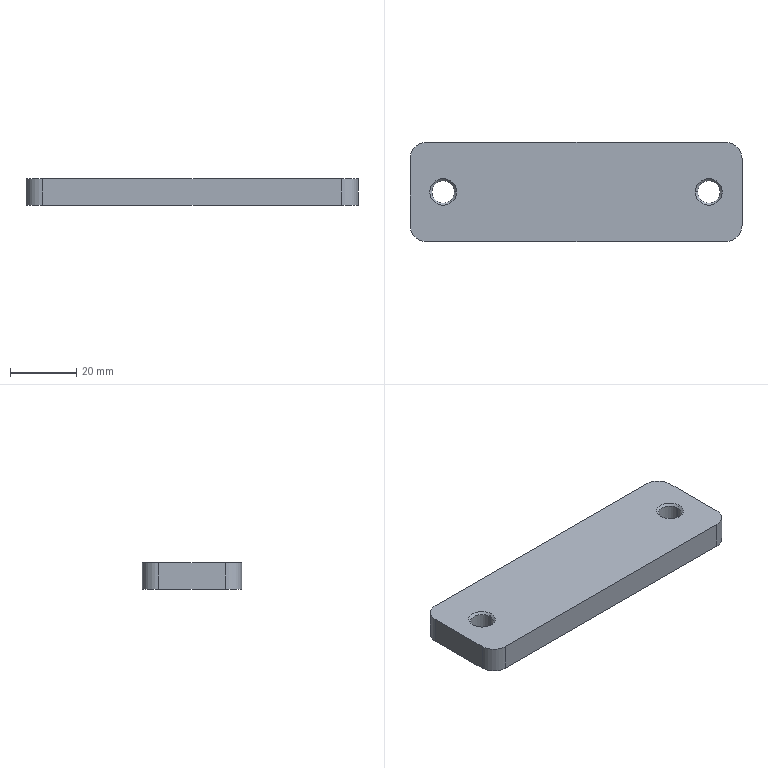Part | SolidWorks | features Extrusion 1, Fillet 1, HoleWzd 1 | 1 solid | 18 faces | box 100 x 30 x 8 mm | volume 23238 mm3 | cylinder 8 | plane 6 | cone 4 | commonest cylinder face diameters 6.8 x4 10 x4
STEP:
#1=CARTESIAN_POINT('',(-43.4,0.,7.375));
#2=VERTEX_POINT('',#1);
#3=CARTESIAN_POINT('',(-36.6,0.,7.375));
#4=VERTEX_POINT('',#3);
#5=CARTESIAN_POINT('',(-40.,0.,7.375));
#6=DIRECTION('',(0.,0.,1.));
#7=DIRECTION('',(1.,0.,0.));
#8=AXIS2_PLACEMENT_3D('',#5,#6,#7);
#9=CIRCLE('',#8,3.4);
#10=EDGE_CURVE('',#2,#4,#9,.T.);
#11=ORIENTED_EDGE('',*,*,#10,.F.);
#12=CARTESIAN_POINT('',(-44.025,0.,8.));
#13=VERTEX_POINT('',#12);
#14=CARTESIAN_POINT('',(-44.025,0.,8.));
#15=DIRECTION('',(-0.7071,0.,0.7071));
#16=VECTOR('',#15,1000.);
#17=LINE('',#14,#16);
#18=EDGE_CURVE('',#2,#13,#17,.T.);
#19=ORIENTED_EDGE('',*,*,#18,.T.);
#20=CARTESIAN_POINT('',(-35.975,0.,8.));
#21=VERTEX_POINT('',#20);
#22=CARTESIAN_POINT('',(-40.,0.,8.));
#23=DIRECTION('',(0.,0.,1.));
#24=DIRECTION('',(1.,0.,0.));
#25=AXIS2_PLACEMENT_3D('',#22,#23,#24);
#26=CIRCLE('',#25,4.025);
#27=EDGE_CURVE('',#13,#21,#26,.T.);
#28=ORIENTED_EDGE('',*,*,#27,.T.);
#29=CARTESIAN_POINT('',(-35.975,0.,8.));
#30=DIRECTION('',(0.7071,0.,0.7071));
#31=VECTOR('',#30,1000.);
#32=LINE('',#29,#31);
#33=EDGE_CURVE('',#4,#21,#32,.T.);
#34=ORIENTED_EDGE('',*,*,#33,.F.);
#35=EDGE_LOOP('',(#11,#19,#28,#34));
#36=FACE_OUTER_BOUND('',#35,.T.);
#37=CARTESIAN_POINT('',(-40.,0.,8.));
#38=DIRECTION('',(0.,0.,1.));
#39=DIRECTION('',(1.,0.,0.));
#40=AXIS2_PLACEMENT_3D('',#37,#38,#39);
#41=CONICAL_SURFACE('',#40,4.025,0.7854);
#42=ADVANCED_FACE('',(#36),#41,.F.);
#43=CARTESIAN_POINT('',(-43.4,0.,0.));
#44=VERTEX_POINT('',#43);
#45=CARTESIAN_POINT('',(-36.6,0.,0.));
#46=VERTEX_POINT('',#45);
#47=CARTESIAN_POINT('',(-40.,0.,0.));
#48=DIRECTION('',(0.,0.,1.));
#49=DIRECTION('',(1.,0.,0.));
#50=AXIS2_PLACEMENT_3D('',#47,#48,#49);
#51=CIRCLE('',#50,3.4);
#52=EDGE_CURVE('',#44,#46,#51,.T.);
#53=ORIENTED_EDGE('',*,*,#52,.F.);
#54=CARTESIAN_POINT('',(-43.4,0.,8.));
#55=DIRECTION('',(0.,0.,1.));
#56=VECTOR('',#55,1000.);
#57=LINE('',#54,#56);
#58=EDGE_CURVE('',#44,#2,#57,.T.);
#59=ORIENTED_EDGE('',*,*,#58,.T.);
#60=ORIENTED_EDGE('',*,*,#10,.T.);
#61=CARTESIAN_POINT('',(-36.6,0.,8.));
#62=DIRECTION('',(0.,0.,1.));
#63=VECTOR('',#62,1000.);
#64=LINE('',#61,#63);
#65=EDGE_CURVE('',#46,#4,#64,.T.);
#66=ORIENTED_EDGE('',*,*,#65,.F.);
#67=EDGE_LOOP('',(#53,#59,#60,#66));
#68=FACE_OUTER_BOUND('',#67,.T.);
#69=CARTESIAN_POINT('',(-40.,0.,8.));
#70=DIRECTION('',(0.,0.,1.));
#71=DIRECTION('',(1.,0.,0.));
#72=AXIS2_PLACEMENT_3D('',#69,#70,#71);
#73=CYLINDRICAL_SURFACE('',#72,3.4);
#74=ADVANCED_FACE('',(#68),#73,.F.);
#75=CARTESIAN_POINT('',(36.6,0.,7.375));
#76=VERTEX_POINT('',#75);
#77=CARTESIAN_POINT('',(43.4,0.,7.375));
#78=VERTEX_POINT('',#77);
#79=CARTESIAN_POINT('',(40.,0.,7.375));
#80=DIRECTION('',(0.,0.,1.));
#81=DIRECTION('',(1.,0.,0.));
#82=AXIS2_PLACEMENT_3D('',#79,#80,#81);
#83=CIRCLE('',#82,3.4);
#84=EDGE_CURVE('',#76,#78,#83,.T.);
#85=ORIENTED_EDGE('',*,*,#84,.F.);
#86=CARTESIAN_POINT('',(35.975,0.,8.));
#87=VERTEX_POINT('',#86);
#88=CARTESIAN_POINT('',(35.975,0.,8.));
#89=DIRECTION('',(-0.7071,0.,0.7071));
#90=VECTOR('',#89,1000.);
#91=LINE('',#88,#90);
#92=EDGE_CURVE('',#76,#87,#91,.T.);
#93=ORIENTED_EDGE('',*,*,#92,.T.);
#94=CARTESIAN_POINT('',(44.025,0.,8.));
#95=VERTEX_POINT('',#94);
#96=CARTESIAN_POINT('',(40.,0.,8.));
#97=DIRECTION('',(0.,0.,1.));
#98=DIRECTION('',(1.,0.,0.));
#99=AXIS2_PLACEMENT_3D('',#96,#97,#98);
#100=CIRCLE('',#99,4.025);
#101=EDGE_CURVE('',#87,#95,#100,.T.);
#102=ORIENTED_EDGE('',*,*,#101,.T.);
#103=CARTESIAN_POINT('',(44.025,0.,8.));
#104=DIRECTION('',(0.7071,0.,0.7071));
#105=VECTOR('',#104,1000.);
#106=LINE('',#103,#105);
#107=EDGE_CURVE('',#78,#95,#106,.T.);
#108=ORIENTED_EDGE('',*,*,#107,.F.);
#109=EDGE_LOOP('',(#85,#93,#102,#108));
#110=FACE_OUTER_BOUND('',#109,.T.);
#111=CARTESIAN_POINT('',(40.,0.,8.));
#112=DIRECTION('',(0.,0.,1.));
#113=DIRECTION('',(1.,0.,0.));
#114=AXIS2_PLACEMENT_3D('',#111,#112,#113);
#115=CONICAL_SURFACE('',#114,4.025,0.7854);
#116=ADVANCED_FACE('',(#110),#115,.F.);
#117=CARTESIAN_POINT('',(36.6,0.,0.));
#118=VERTEX_POINT('',#117);
#119=CARTESIAN_POINT('',(43.4,0.,0.));
#120=VERTEX_POINT('',#119);
#121=CARTESIAN_POINT('',(40.,0.,0.));
#122=DIRECTION('',(0.,0.,1.));
#123=DIRECTION('',(1.,0.,0.));
#124=AXIS2_PLACEMENT_3D('',#121,#122,#123);
#125=CIRCLE('',#124,3.4);
#126=EDGE_CURVE('',#118,#120,#125,.T.);
#127=ORIENTED_EDGE('',*,*,#126,.F.);
#128=CARTESIAN_POINT('',(36.6,0.,8.));
#129=DIRECTION('',(0.,0.,1.));
#130=VECTOR('',#129,1000.);
#131=LINE('',#128,#130);
#132=EDGE_CURVE('',#118,#76,#131,.T.);
#133=ORIENTED_EDGE('',*,*,#132,.T.);
#134=ORIENTED_EDGE('',*,*,#84,.T.);
#135=CARTESIAN_POINT('',(43.4,0.,8.));
#136=DIRECTION('',(0.,0.,1.));
#137=VECTOR('',#136,1000.);
#138=LINE('',#135,#137);
#139=EDGE_CURVE('',#120,#78,#138,.T.);
#140=ORIENTED_EDGE('',*,*,#139,.F.);
#141=EDGE_LOOP('',(#127,#133,#134,#140));
#142=FACE_OUTER_BOUND('',#141,.T.);
#143=CARTESIAN_POINT('',(40.,0.,8.));
#144=DIRECTION('',(0.,0.,1.));
#145=DIRECTION('',(1.,0.,0.));
#146=AXIS2_PLACEMENT_3D('',#143,#144,#145);
#147=CYLINDRICAL_SURFACE('',#146,3.4);
#148=ADVANCED_FACE('',(#142),#147,.F.);
#149=CARTESIAN_POINT('',(50.,-10.,8.));
#150=VERTEX_POINT('',#149);
#151=CARTESIAN_POINT('',(50.,10.,8.));
#152=VERTEX_POINT('',#151);
#153=CARTESIAN_POINT('',(50.,-15.,8.));
#154=DIRECTION('',(0.,1.,0.));
#155=VECTOR('',#154,1000.);
#156=LINE('',#153,#155);
#157=EDGE_CURVE('',#150,#152,#156,.T.);
#158=ORIENTED_EDGE('',*,*,#157,.F.);
#159=CARTESIAN_POINT('',(50.,-10.,0.));
#160=VERTEX_POINT('',#159);
#161=CARTESIAN_POINT('',(50.,-10.,8.));
#162=DIRECTION('',(0.,0.,-1.));
#163=VECTOR('',#162,1000.);
#164=LINE('',#161,#163);
#165=EDGE_CURVE('',#150,#160,#164,.T.);
#166=ORIENTED_EDGE('',*,*,#165,.T.);
#167=CARTESIAN_POINT('',(50.,10.,0.));
#168=VERTEX_POINT('',#167);
#169=CARTESIAN_POINT('',(50.,-15.,0.));
#170=DIRECTION('',(0.,1.,0.));
#171=VECTOR('',#170,1000.);
#172=LINE('',#169,#171);
#173=EDGE_CURVE('',#160,#168,#172,.T.);
#174=ORIENTED_EDGE('',*,*,#173,.T.);
#175=CARTESIAN_POINT('',(50.,10.,8.));
#176=DIRECTION('',(0.,0.,1.));
#177=VECTOR('',#176,1000.);
#178=LINE('',#175,#177);
#179=EDGE_CURVE('',#168,#152,#178,.T.);
#180=ORIENTED_EDGE('',*,*,#179,.T.);
#181=EDGE_LOOP('',(#158,#166,#174,#180));
#182=FACE_OUTER_BOUND('',#181,.T.);
#183=CARTESIAN_POINT('',(50.,-15.,8.));
#184=DIRECTION('',(-1.,0.,0.));
#185=DIRECTION('',(0.,0.,1.));
#186=AXIS2_PLACEMENT_3D('',#183,#184,#185);
#187=PLANE('',#186);
#188=ADVANCED_FACE('',(#182),#187,.F.);
#189=CARTESIAN_POINT('',(45.,15.,8.));
#190=VERTEX_POINT('',#189);
#191=CARTESIAN_POINT('',(-45.,15.,8.));
#192=VERTEX_POINT('',#191);
#193=CARTESIAN_POINT('',(-50.,15.,8.));
#194=DIRECTION('',(-1.,0.,0.));
#195=VECTOR('',#194,1000.);
#196=LINE('',#193,#195);
#197=EDGE_CURVE('',#190,#192,#196,.T.);
#198=ORIENTED_EDGE('',*,*,#197,.F.);
#199=CARTESIAN_POINT('',(45.,15.,0.));
#200=VERTEX_POINT('',#199);
#201=CARTESIAN_POINT('',(45.,15.,8.));
#202=DIRECTION('',(0.,0.,-1.));
#203=VECTOR('',#202,1000.);
#204=LINE('',#201,#203);
#205=EDGE_CURVE('',#190,#200,#204,.T.);
#206=ORIENTED_EDGE('',*,*,#205,.T.);
#207=CARTESIAN_POINT('',(-45.,15.,0.));
#208=VERTEX_POINT('',#207);
#209=CARTESIAN_POINT('',(-50.,15.,0.));
#210=DIRECTION('',(-1.,0.,0.));
#211=VECTOR('',#210,1000.);
#212=LINE('',#209,#211);
#213=EDGE_CURVE('',#200,#208,#212,.T.);
#214=ORIENTED_EDGE('',*,*,#213,.T.);
#215=CARTESIAN_POINT('',(-45.,15.,8.));
#216=DIRECTION('',(0.,0.,1.));
#217=VECTOR('',#216,1000.);
#218=LINE('',#215,#217);
#219=EDGE_CURVE('',#208,#192,#218,.T.);
#220=ORIENTED_EDGE('',*,*,#219,.T.);
#221=EDGE_LOOP('',(#198,#206,#214,#220));
#222=FACE_OUTER_BOUND('',#221,.T.);
#223=CARTESIAN_POINT('',(-50.,15.,8.));
#224=DIRECTION('',(0.,-1.,0.));
#225=DIRECTION('',(0.,0.,-1.));
#226=AXIS2_PLACEMENT_3D('',#223,#224,#225);
#227=PLANE('',#226);
#228=ADVANCED_FACE('',(#222),#227,.F.);
#229=CARTESIAN_POINT('',(-50.,10.,0.));
#230=VERTEX_POINT('',#229);
#231=CARTESIAN_POINT('',(-50.,-10.,0.));
#232=VERTEX_POINT('',#231);
#233=CARTESIAN_POINT('',(-50.,-15.,0.));
#234=DIRECTION('',(0.,-1.,0.));
#235=VECTOR('',#234,1000.);
#236=LINE('',#233,#235);
#237=EDGE_CURVE('',#230,#232,#236,.T.);
#238=ORIENTED_EDGE('',*,*,#237,.T.);
#239=CARTESIAN_POINT('',(-50.,-10.,8.));
#240=VERTEX_POINT('',#239);
#241=CARTESIAN_POINT('',(-50.,-10.,8.));
#242=DIRECTION('',(0.,0.,1.));
#243=VECTOR('',#242,1000.);
#244=LINE('',#241,#243);
#245=EDGE_CURVE('',#232,#240,#244,.T.);
#246=ORIENTED_EDGE('',*,*,#245,.T.);
#247=CARTESIAN_POINT('',(-50.,10.,8.));
#248=VERTEX_POINT('',#247);
#249=CARTESIAN_POINT('',(-50.,-15.,8.));
#250=DIRECTION('',(0.,-1.,0.));
#251=VECTOR('',#250,1000.);
#252=LINE('',#249,#251);
#253=EDGE_CURVE('',#248,#240,#252,.T.);
#254=ORIENTED_EDGE('',*,*,#253,.F.);
#255=CARTESIAN_POINT('',(-50.,10.,8.));
#256=DIRECTION('',(0.,0.,-1.));
#257=VECTOR('',#256,1000.);
#258=LINE('',#255,#257);
#259=EDGE_CURVE('',#248,#230,#258,.T.);
#260=ORIENTED_EDGE('',*,*,#259,.T.);
#261=EDGE_LOOP('',(#238,#246,#254,#260));
#262=FACE_OUTER_BOUND('',#261,.T.);
#263=CARTESIAN_POINT('',(-50.,-15.,8.));
#264=DIRECTION('',(1.,0.,0.));
#265=DIRECTION('',(0.,0.,-1.));
#266=AXIS2_PLACEMENT_3D('',#263,#264,#265);
#267=PLANE('',#266);
#268=ADVANCED_FACE('',(#262),#267,.F.);
#269=CARTESIAN_POINT('',(-45.,-15.,0.));
#270=VERTEX_POINT('',#269);
#271=CARTESIAN_POINT('',(45.,-15.,0.));
#272=VERTEX_POINT('',#271);
#273=CARTESIAN_POINT('',(-50.,-15.,0.));
#274=DIRECTION('',(1.,0.,0.));
#275=VECTOR('',#274,1000.);
#276=LINE('',#273,#275);
#277=EDGE_CURVE('',#270,#272,#276,.T.);
#278=ORIENTED_EDGE('',*,*,#277,.T.);
#279=CARTESIAN_POINT('',(45.,-15.,8.));
#280=VERTEX_POINT('',#279);
#281=CARTESIAN_POINT('',(45.,-15.,8.));
#282=DIRECTION('',(0.,0.,1.));
#283=VECTOR('',#282,1000.);
#284=LINE('',#281,#283);
#285=EDGE_CURVE('',#272,#280,#284,.T.);
#286=ORIENTED_EDGE('',*,*,#285,.T.);
#287=CARTESIAN_POINT('',(-45.,-15.,8.));
#288=VERTEX_POINT('',#287);
#289=CARTESIAN_POINT('',(-50.,-15.,8.));
#290=DIRECTION('',(1.,0.,0.));
#291=VECTOR('',#290,1000.);
#292=LINE('',#289,#291);
#293=EDGE_CURVE('',#288,#280,#292,.T.);
#294=ORIENTED_EDGE('',*,*,#293,.F.);
#295=CARTESIAN_POINT('',(-45.,-15.,8.));
#296=DIRECTION('',(0.,0.,-1.));
#297=VECTOR('',#296,1000.);
#298=LINE('',#295,#297);
#299=EDGE_CURVE('',#288,#270,#298,.T.);
#300=ORIENTED_EDGE('',*,*,#299,.T.);
#301=EDGE_LOOP('',(#278,#286,#294,#300));
#302=FACE_OUTER_BOUND('',#301,.T.);
#303=CARTESIAN_POINT('',(-50.,-15.,8.));
#304=DIRECTION('',(0.,1.,0.));
#305=DIRECTION('',(0.,0.,1.));
#306=AXIS2_PLACEMENT_3D('',#303,#304,#305);
#307=PLANE('',#306);
#308=ADVANCED_FACE('',(#302),#307,.F.);
#309=CARTESIAN_POINT('',(-40.,0.,8.));
#310=DIRECTION('',(0.,0.,1.));
#311=DIRECTION('',(1.,0.,0.));
#312=AXIS2_PLACEMENT_3D('',#309,#310,#311);
#313=CIRCLE('',#312,4.025);
#314=EDGE_CURVE('',#21,#13,#313,.T.);
#315=ORIENTED_EDGE('',*,*,#314,.F.);
#316=ORIENTED_EDGE('',*,*,#27,.F.);
#317=EDGE_LOOP('',(#315,#316));
#318=FACE_BOUND('',#317,.T.);
#319=CARTESIAN_POINT('',(40.,0.,8.));
#320=DIRECTION('',(0.,0.,1.));
#321=DIRECTION('',(1.,0.,0.));
#322=AXIS2_PLACEMENT_3D('',#319,#320,#321);
#323=CIRCLE('',#322,4.025);
#324=EDGE_CURVE('',#95,#87,#323,.T.);
#325=ORIENTED_EDGE('',*,*,#324,.F.);
#326=ORIENTED_EDGE('',*,*,#101,.F.);
#327=EDGE_LOOP('',(#325,#326));
#328=FACE_BOUND('',#327,.T.);
#329=ORIENTED_EDGE('',*,*,#293,.T.);
#330=CARTESIAN_POINT('',(45.,-10.,8.));
#331=DIRECTION('',(0.,0.,1.));
#332=DIRECTION('',(-1.,0.,0.));
#333=AXIS2_PLACEMENT_3D('',#330,#331,#332);
#334=CIRCLE('',#333,5.);
#335=EDGE_CURVE('',#280,#150,#334,.T.);
#336=ORIENTED_EDGE('',*,*,#335,.T.);
#337=ORIENTED_EDGE('',*,*,#157,.T.);
#338=CARTESIAN_POINT('',(45.,10.,8.));
#339=DIRECTION('',(0.,0.,1.));
#340=DIRECTION('',(-1.,0.,0.));
#341=AXIS2_PLACEMENT_3D('',#338,#339,#340);
#342=CIRCLE('',#341,5.);
#343=EDGE_CURVE('',#152,#190,#342,.T.);
#344=ORIENTED_EDGE('',*,*,#343,.T.);
#345=ORIENTED_EDGE('',*,*,#197,.T.);
#346=CARTESIAN_POINT('',(-45.,10.,8.));
#347=DIRECTION('',(0.,0.,1.));
#348=DIRECTION('',(-1.,0.,0.));
#349=AXIS2_PLACEMENT_3D('',#346,#347,#348);
#350=CIRCLE('',#349,5.);
#351=EDGE_CURVE('',#192,#248,#350,.T.);
#352=ORIENTED_EDGE('',*,*,#351,.T.);
#353=ORIENTED_EDGE('',*,*,#253,.T.);
#354=CARTESIAN_POINT('',(-45.,-10.,8.));
#355=DIRECTION('',(0.,0.,1.));
#356=DIRECTION('',(-1.,0.,0.));
#357=AXIS2_PLACEMENT_3D('',#354,#355,#356);
#358=CIRCLE('',#357,5.);
#359=EDGE_CURVE('',#240,#288,#358,.T.);
#360=ORIENTED_EDGE('',*,*,#359,.T.);
#361=EDGE_LOOP('',(#329,#336,#337,#344,#345,#352,#353,#360));
#362=FACE_OUTER_BOUND('',#361,.T.);
#363=CARTESIAN_POINT('',(0.,0.,8.));
#364=DIRECTION('',(0.,0.,-1.));
#365=DIRECTION('',(-1.,0.,0.));
#366=AXIS2_PLACEMENT_3D('',#363,#364,#365);
#367=PLANE('',#366);
#368=ADVANCED_FACE('',(#318,#328,#362),#367,.F.);
#369=CARTESIAN_POINT('',(-40.,0.,0.));
#370=DIRECTION('',(0.,0.,1.));
#371=DIRECTION('',(1.,0.,0.));
#372=AXIS2_PLACEMENT_3D('',#369,#370,#371);
#373=CIRCLE('',#372,3.4);
#374=EDGE_CURVE('',#46,#44,#373,.T.);
#375=ORIENTED_EDGE('',*,*,#374,.T.);
#376=ORIENTED_EDGE('',*,*,#52,.T.);
#377=EDGE_LOOP('',(#375,#376));
#378=FACE_BOUND('',#377,.T.);
#379=CARTESIAN_POINT('',(40.,0.,0.));
#380=DIRECTION('',(0.,0.,1.));
#381=DIRECTION('',(1.,0.,0.));
#382=AXIS2_PLACEMENT_3D('',#379,#380,#381);
#383=CIRCLE('',#382,3.4);
#384=EDGE_CURVE('',#120,#118,#383,.T.);
#385=ORIENTED_EDGE('',*,*,#384,.T.);
#386=ORIENTED_EDGE('',*,*,#126,.T.);
#387=EDGE_LOOP('',(#385,#386));
#388=FACE_BOUND('',#387,.T.);
#389=ORIENTED_EDGE('',*,*,#173,.F.);
#390=CARTESIAN_POINT('',(45.,-10.,0.));
#391=DIRECTION('',(0.,0.,-1.));
#392=DIRECTION('',(-1.,0.,0.));
#393=AXIS2_PLACEMENT_3D('',#390,#391,#392);
#394=CIRCLE('',#393,5.);
#395=EDGE_CURVE('',#160,#272,#394,.T.);
#396=ORIENTED_EDGE('',*,*,#395,.T.);
#397=ORIENTED_EDGE('',*,*,#277,.F.);
#398=CARTESIAN_POINT('',(-45.,-10.,0.));
#399=DIRECTION('',(0.,0.,-1.));
#400=DIRECTION('',(-1.,0.,0.));
#401=AXIS2_PLACEMENT_3D('',#398,#399,#400);
#402=CIRCLE('',#401,5.);
#403=EDGE_CURVE('',#270,#232,#402,.T.);
#404=ORIENTED_EDGE('',*,*,#403,.T.);
#405=ORIENTED_EDGE('',*,*,#237,.F.);
#406=CARTESIAN_POINT('',(-45.,10.,0.));
#407=DIRECTION('',(0.,0.,-1.));
#408=DIRECTION('',(-1.,0.,0.));
#409=AXIS2_PLACEMENT_3D('',#406,#407,#408);
#410=CIRCLE('',#409,5.);
#411=EDGE_CURVE('',#230,#208,#410,.T.);
#412=ORIENTED_EDGE('',*,*,#411,.T.);
#413=ORIENTED_EDGE('',*,*,#213,.F.);
#414=CARTESIAN_POINT('',(45.,10.,0.));
#415=DIRECTION('',(0.,0.,-1.));
#416=DIRECTION('',(-1.,0.,0.));
#417=AXIS2_PLACEMENT_3D('',#414,#415,#416);
#418=CIRCLE('',#417,5.);
#419=EDGE_CURVE('',#200,#168,#418,.T.);
#420=ORIENTED_EDGE('',*,*,#419,.T.);
#421=EDGE_LOOP('',(#389,#396,#397,#404,#405,#412,#413,#420));
#422=FACE_OUTER_BOUND('',#421,.T.);
#423=CARTESIAN_POINT('',(0.,0.,0.));
#424=DIRECTION('',(0.,0.,-1.));
#425=DIRECTION('',(-1.,0.,0.));
#426=AXIS2_PLACEMENT_3D('',#423,#424,#425);
#427=PLANE('',#426);
#428=ADVANCED_FACE('',(#378,#388,#422),#427,.T.);
#429=ORIENTED_EDGE('',*,*,#335,.F.);
#430=ORIENTED_EDGE('',*,*,#285,.F.);
#431=ORIENTED_EDGE('',*,*,#395,.F.);
#432=ORIENTED_EDGE('',*,*,#165,.F.);
#433=EDGE_LOOP('',(#429,#430,#431,#432));
#434=FACE_OUTER_BOUND('',#433,.T.);
#435=CARTESIAN_POINT('',(45.,-10.,8.));
#436=DIRECTION('',(0.,0.,-1.));
#437=DIRECTION('',(-1.,0.,0.));
#438=AXIS2_PLACEMENT_3D('',#435,#436,#437);
#439=CYLINDRICAL_SURFACE('',#438,5.);
#440=ADVANCED_FACE('',(#434),#439,.T.);
#441=ORIENTED_EDGE('',*,*,#343,.F.);
#442=ORIENTED_EDGE('',*,*,#179,.F.);
#443=ORIENTED_EDGE('',*,*,#419,.F.);
#444=ORIENTED_EDGE('',*,*,#205,.F.);
#445=EDGE_LOOP('',(#441,#442,#443,#444));
#446=FACE_OUTER_BOUND('',#445,.T.);
#447=CARTESIAN_POINT('',(45.,10.,8.));
#448=DIRECTION('',(0.,0.,-1.));
#449=DIRECTION('',(-1.,0.,0.));
#450=AXIS2_PLACEMENT_3D('',#447,#448,#449);
#451=CYLINDRICAL_SURFACE('',#450,5.);
#452=ADVANCED_FACE('',(#446),#451,.T.);
#453=ORIENTED_EDGE('',*,*,#359,.F.);
#454=ORIENTED_EDGE('',*,*,#245,.F.);
#455=ORIENTED_EDGE('',*,*,#403,.F.);
#456=ORIENTED_EDGE('',*,*,#299,.F.);
#457=EDGE_LOOP('',(#453,#454,#455,#456));
#458=FACE_OUTER_BOUND('',#457,.T.);
#459=CARTESIAN_POINT('',(-45.,-10.,8.));
#460=DIRECTION('',(0.,0.,-1.));
#461=DIRECTION('',(-1.,0.,0.));
#462=AXIS2_PLACEMENT_3D('',#459,#460,#461);
#463=CYLINDRICAL_SURFACE('',#462,5.);
#464=ADVANCED_FACE('',(#458),#463,.T.);
#465=ORIENTED_EDGE('',*,*,#351,.F.);
#466=ORIENTED_EDGE('',*,*,#219,.F.);
#467=ORIENTED_EDGE('',*,*,#411,.F.);
#468=ORIENTED_EDGE('',*,*,#259,.F.);
#469=EDGE_LOOP('',(#465,#466,#467,#468));
#470=FACE_OUTER_BOUND('',#469,.T.);
#471=CARTESIAN_POINT('',(-45.,10.,8.));
#472=DIRECTION('',(0.,0.,-1.));
#473=DIRECTION('',(-1.,0.,0.));
#474=AXIS2_PLACEMENT_3D('',#471,#472,#473);
#475=CYLINDRICAL_SURFACE('',#474,5.);
#476=ADVANCED_FACE('',(#470),#475,.T.);
#477=ORIENTED_EDGE('',*,*,#132,.F.);
#478=ORIENTED_EDGE('',*,*,#384,.F.);
#479=ORIENTED_EDGE('',*,*,#139,.T.);
#480=CARTESIAN_POINT('',(40.,0.,7.375));
#481=DIRECTION('',(0.,0.,1.));
#482=DIRECTION('',(1.,0.,0.));
#483=AXIS2_PLACEMENT_3D('',#480,#481,#482);
#484=CIRCLE('',#483,3.4);
#485=EDGE_CURVE('',#78,#76,#484,.T.);
#486=ORIENTED_EDGE('',*,*,#485,.T.);
#487=EDGE_LOOP('',(#477,#478,#479,#486));
#488=FACE_OUTER_BOUND('',#487,.T.);
#489=CARTESIAN_POINT('',(40.,0.,8.));
#490=DIRECTION('',(0.,0.,1.));
#491=DIRECTION('',(1.,0.,0.));
#492=AXIS2_PLACEMENT_3D('',#489,#490,#491);
#493=CYLINDRICAL_SURFACE('',#492,3.4);
#494=ADVANCED_FACE('',(#488),#493,.F.);
#495=ORIENTED_EDGE('',*,*,#92,.F.);
#496=ORIENTED_EDGE('',*,*,#485,.F.);
#497=ORIENTED_EDGE('',*,*,#107,.T.);
#498=ORIENTED_EDGE('',*,*,#324,.T.);
#499=EDGE_LOOP('',(#495,#496,#497,#498));
#500=FACE_OUTER_BOUND('',#499,.T.);
#501=CARTESIAN_POINT('',(40.,0.,8.));
#502=DIRECTION('',(0.,0.,1.));
#503=DIRECTION('',(1.,0.,0.));
#504=AXIS2_PLACEMENT_3D('',#501,#502,#503);
#505=CONICAL_SURFACE('',#504,4.025,0.7854);
#506=ADVANCED_FACE('',(#500),#505,.F.);
#507=ORIENTED_EDGE('',*,*,#58,.F.);
#508=ORIENTED_EDGE('',*,*,#374,.F.);
#509=ORIENTED_EDGE('',*,*,#65,.T.);
#510=CARTESIAN_POINT('',(-40.,0.,7.375));
#511=DIRECTION('',(0.,0.,1.));
#512=DIRECTION('',(1.,0.,0.));
#513=AXIS2_PLACEMENT_3D('',#510,#511,#512);
#514=CIRCLE('',#513,3.4);
#515=EDGE_CURVE('',#4,#2,#514,.T.);
#516=ORIENTED_EDGE('',*,*,#515,.T.);
#517=EDGE_LOOP('',(#507,#508,#509,#516));
#518=FACE_OUTER_BOUND('',#517,.T.);
#519=CARTESIAN_POINT('',(-40.,0.,8.));
#520=DIRECTION('',(0.,0.,1.));
#521=DIRECTION('',(1.,0.,0.));
#522=AXIS2_PLACEMENT_3D('',#519,#520,#521);
#523=CYLINDRICAL_SURFACE('',#522,3.4);
#524=ADVANCED_FACE('',(#518),#523,.F.);
#525=ORIENTED_EDGE('',*,*,#18,.F.);
#526=ORIENTED_EDGE('',*,*,#515,.F.);
#527=ORIENTED_EDGE('',*,*,#33,.T.);
#528=ORIENTED_EDGE('',*,*,#314,.T.);
#529=EDGE_LOOP('',(#525,#526,#527,#528));
#530=FACE_OUTER_BOUND('',#529,.T.);
#531=CARTESIAN_POINT('',(-40.,0.,8.));
#532=DIRECTION('',(0.,0.,1.));
#533=DIRECTION('',(1.,0.,0.));
#534=AXIS2_PLACEMENT_3D('',#531,#532,#533);
#535=CONICAL_SURFACE('',#534,4.025,0.7854);
#536=ADVANCED_FACE('',(#530),#535,.F.);
#537=CLOSED_SHELL('',(#42,#74,#116,#148,#188,#228,#268,#308,#368,#428,#440,#452,#464,#476,#494,#506,#524,#536));
#538=MANIFOLD_SOLID_BREP('',#537);
#539=CARTESIAN_POINT('',(0.,0.,0.));
#540=DIRECTION('',(0.,0.,1.));
#541=DIRECTION('',(1.,0.,0.));
#542=AXIS2_PLACEMENT_3D('',#539,#540,#541);
#543=(LENGTH_UNIT()NAMED_UNIT(*)SI_UNIT(.MILLI.,.METRE.));
#544=UNCERTAINTY_MEASURE_WITH_UNIT(LENGTH_MEASURE(0.00001),#543,'','');
#545=(NAMED_UNIT(*)PLANE_ANGLE_UNIT()SI_UNIT($,.RADIAN.));
#546=(NAMED_UNIT(*)SI_UNIT($,.STERADIAN.)SOLID_ANGLE_UNIT());
#547=(GEOMETRIC_REPRESENTATION_CONTEXT(3)GLOBAL_UNCERTAINTY_ASSIGNED_CONTEXT((#544))GLOBAL_UNIT_ASSIGNED_CONTEXT((#543,#545,#546))REPRESENTATION_CONTEXT('',''));
#548=ADVANCED_BREP_SHAPE_REPRESENTATION('',(#538,#542),#547);